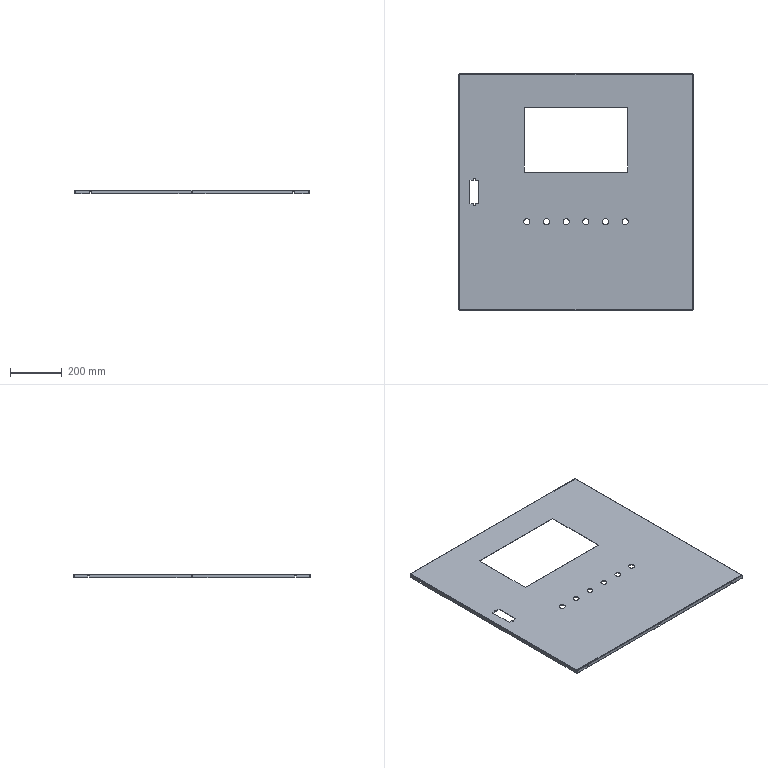Part | SolidWorks | features ICE 5, EdgeFlange 1, FlatPattern 1, LPattern 1, SMBaseFlange 1, SheetMetal 1 | 1 solid | 126 faces | box 905 x 915 x 15 mm | volume 1150481 mm3 | plane 72 | cylinder 46 | spline 8 | commonest cylinder face diameters 7 x26 23 x12 2 x4 5 x4